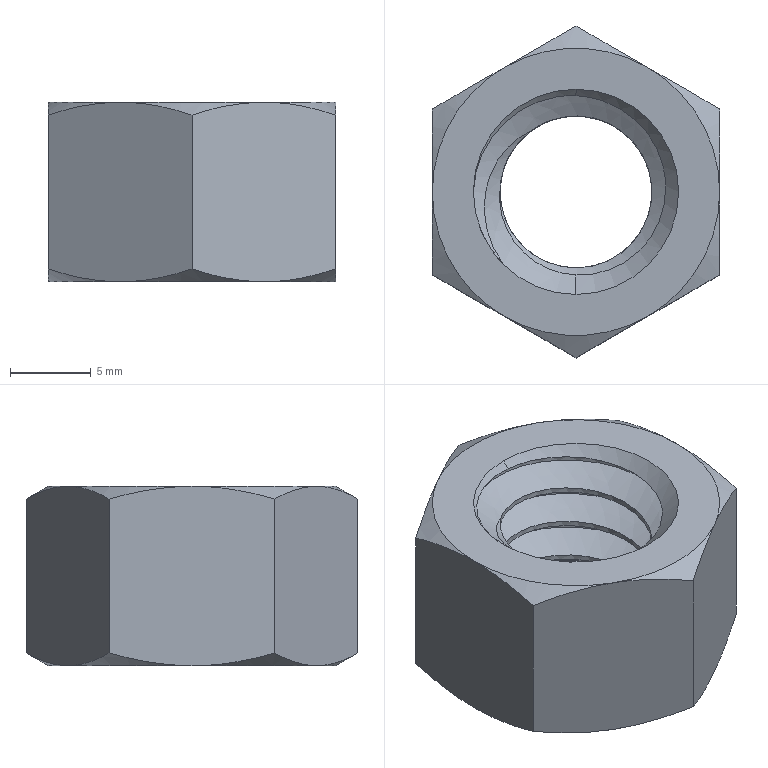Part | SolidWorks | features Extrusion 1, Helix 1, ICE 1, MirrorPattern 1, RevCut 1, Scale 1, Sweep 1 | 1 solid | 39 faces | box 17.78 x 20.531 x 11.113 mm | volume 1918 mm3 | cone 18 | cylinder 10 | plane 8 | spline 3 | commonest cylinder face diameters 12.7 x10